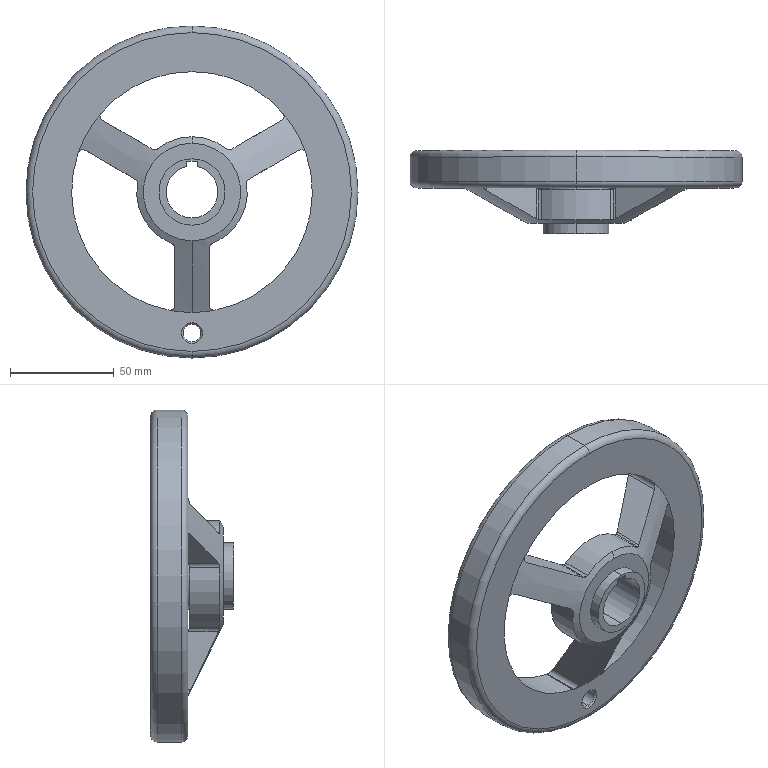Part | SolidWorks | features ICE 4, MBimport 1 | 1 solid | 64 faces | box 160 x 40 x 160 mm | volume 222311 mm3 | cylinder 36 | plane 16 | cone 8 | torus 4 | commonest cylinder face diameters 4.571 x16 32 x4 53.333 x3 116 x3 8.376 x2 25 x2